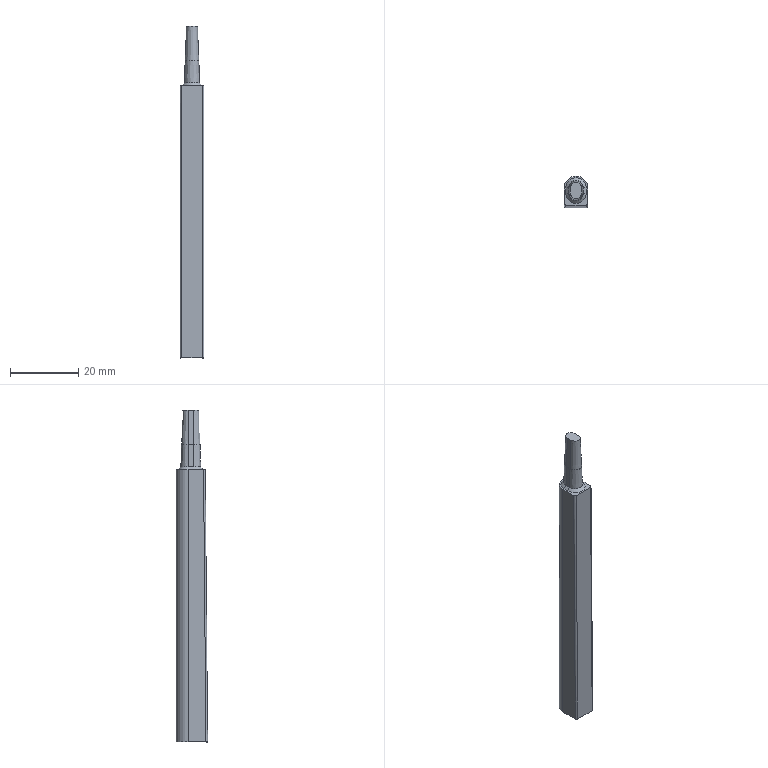Part | SolidWorks | features BaseBody 1 | 1 solid | 22 faces | box 7 x 9.198 x 97.496 mm | volume 4841 mm3 | plane 13 | cone 6 | cylinder 3 | commonest cylinder face diameters 1 x2 7 x1
STEP:
#1=CARTESIAN_POINT('',(-166.55,-32.434,17.496));
#2=VERTEX_POINT('',#1);
#3=CARTESIAN_POINT('',(-169.79,-32.434,17.496));
#4=VERTEX_POINT('',#3);
#5=CARTESIAN_POINT('',(-168.17,-32.434,17.496));
#6=DIRECTION('',(0.,0.,1.));
#7=DIRECTION('',(1.,0.,0.));
#8=AXIS2_PLACEMENT_3D('',#5,#6,#7);
#9=CIRCLE('',#8,1.62);
#10=EDGE_CURVE('',#2,#4,#9,.T.);
#11=ORIENTED_EDGE('',*,*,#10,.T.);
#12=CARTESIAN_POINT('',(-169.79,-33.942,17.496));
#13=VERTEX_POINT('',#12);
#14=CARTESIAN_POINT('',(-169.79,-33.188,17.496));
#15=DIRECTION('',(0.,-1.,0.));
#16=VECTOR('',#15,1000.);
#17=LINE('',#14,#16);
#18=EDGE_CURVE('',#4,#13,#17,.T.);
#19=ORIENTED_EDGE('',*,*,#18,.T.);
#20=CARTESIAN_POINT('',(-166.55,-33.942,17.496));
#21=VERTEX_POINT('',#20);
#22=CARTESIAN_POINT('',(-168.17,-33.942,17.496));
#23=DIRECTION('',(0.,0.,1.));
#24=DIRECTION('',(1.,0.,0.));
#25=AXIS2_PLACEMENT_3D('',#22,#23,#24);
#26=CIRCLE('',#25,1.62);
#27=EDGE_CURVE('',#13,#21,#26,.T.);
#28=ORIENTED_EDGE('',*,*,#27,.T.);
#29=CARTESIAN_POINT('',(-166.55,-33.188,17.496));
#30=DIRECTION('',(0.,1.,0.));
#31=VECTOR('',#30,1000.);
#32=LINE('',#29,#31);
#33=EDGE_CURVE('',#21,#2,#32,.T.);
#34=ORIENTED_EDGE('',*,*,#33,.T.);
#35=EDGE_LOOP('',(#11,#19,#28,#34));
#36=FACE_OUTER_BOUND('',#35,.T.);
#37=CARTESIAN_POINT('',(-178.728,104.314,17.496));
#38=DIRECTION('',(0.,0.,-1.));
#39=DIRECTION('',(1.,0.,0.));
#40=AXIS2_PLACEMENT_3D('',#37,#38,#39);
#41=PLANE('',#40);
#42=ADVANCED_FACE('',(#36),#41,.F.);
#43=CARTESIAN_POINT('',(-166.199,-33.942,7.441));
#44=VERTEX_POINT('',#43);
#45=CARTESIAN_POINT('',(-166.209,-33.942,7.732));
#46=DIRECTION('',(-0.0349,0.,0.9994));
#47=VECTOR('',#46,1000.);
#48=LINE('',#45,#47);
#49=EDGE_CURVE('',#44,#21,#48,.T.);
#50=ORIENTED_EDGE('',*,*,#49,.F.);
#51=CARTESIAN_POINT('',(-166.199,-32.434,7.441));
#52=VERTEX_POINT('',#51);
#53=CARTESIAN_POINT('',(-166.199,104.314,7.441));
#54=DIRECTION('',(0.,-1.,0.));
#55=VECTOR('',#54,1000.);
#56=LINE('',#53,#55);
#57=EDGE_CURVE('',#52,#44,#56,.T.);
#58=ORIENTED_EDGE('',*,*,#57,.F.);
#59=CARTESIAN_POINT('',(-166.209,-32.434,7.732));
#60=DIRECTION('',(-0.0349,0.,0.9994));
#61=VECTOR('',#60,1000.);
#62=LINE('',#59,#61);
#63=EDGE_CURVE('',#52,#2,#62,.T.);
#64=ORIENTED_EDGE('',*,*,#63,.T.);
#65=ORIENTED_EDGE('',*,*,#33,.F.);
#66=EDGE_LOOP('',(#50,#58,#64,#65));
#67=FACE_OUTER_BOUND('',#66,.T.);
#68=CARTESIAN_POINT('',(-166.209,-33.188,7.732));
#69=DIRECTION('',(-0.9994,0.,-0.0349));
#70=DIRECTION('',(0.0349,0.,-0.9994));
#71=AXIS2_PLACEMENT_3D('',#68,#69,#70);
#72=PLANE('',#71);
#73=ADVANCED_FACE('',(#67),#72,.F.);
#74=ORIENTED_EDGE('',*,*,#63,.F.);
#75=CARTESIAN_POINT('',(-170.141,-32.434,7.441));
#76=VERTEX_POINT('',#75);
#77=CARTESIAN_POINT('',(-168.17,-32.434,7.441));
#78=DIRECTION('',(0.,0.,-1.));
#79=DIRECTION('',(1.,0.,0.));
#80=AXIS2_PLACEMENT_3D('',#77,#78,#79);
#81=CIRCLE('',#80,1.971);
#82=EDGE_CURVE('',#76,#52,#81,.T.);
#83=ORIENTED_EDGE('',*,*,#82,.F.);
#84=CARTESIAN_POINT('',(-170.131,-32.434,7.732));
#85=DIRECTION('',(0.0349,0.,0.9994));
#86=VECTOR('',#85,1000.);
#87=LINE('',#84,#86);
#88=EDGE_CURVE('',#76,#4,#87,.T.);
#89=ORIENTED_EDGE('',*,*,#88,.T.);
#90=ORIENTED_EDGE('',*,*,#10,.F.);
#91=EDGE_LOOP('',(#74,#83,#89,#90));
#92=FACE_OUTER_BOUND('',#91,.T.);
#93=CARTESIAN_POINT('',(-168.17,-32.434,7.732));
#94=DIRECTION('',(0.,0.,-1.));
#95=DIRECTION('',(1.,0.,0.));
#96=AXIS2_PLACEMENT_3D('',#93,#94,#95);
#97=CONICAL_SURFACE('',#96,1.961,0.03491);
#98=ADVANCED_FACE('',(#92),#97,.T.);
#99=ORIENTED_EDGE('',*,*,#88,.F.);
#100=CARTESIAN_POINT('',(-170.141,-33.942,7.441));
#101=VERTEX_POINT('',#100);
#102=CARTESIAN_POINT('',(-170.141,104.314,7.441));
#103=DIRECTION('',(0.,1.,0.));
#104=VECTOR('',#103,1000.);
#105=LINE('',#102,#104);
#106=EDGE_CURVE('',#101,#76,#105,.T.);
#107=ORIENTED_EDGE('',*,*,#106,.F.);
#108=CARTESIAN_POINT('',(-170.131,-33.942,7.732));
#109=DIRECTION('',(0.0349,0.,0.9994));
#110=VECTOR('',#109,1000.);
#111=LINE('',#108,#110);
#112=EDGE_CURVE('',#101,#13,#111,.T.);
#113=ORIENTED_EDGE('',*,*,#112,.T.);
#114=ORIENTED_EDGE('',*,*,#18,.F.);
#115=EDGE_LOOP('',(#99,#107,#113,#114));
#116=FACE_OUTER_BOUND('',#115,.T.);
#117=CARTESIAN_POINT('',(-170.131,-33.188,7.732));
#118=DIRECTION('',(0.9994,0.,-0.0349));
#119=DIRECTION('',(0.0349,0.,0.9994));
#120=AXIS2_PLACEMENT_3D('',#117,#118,#119);
#121=PLANE('',#120);
#122=ADVANCED_FACE('',(#116),#121,.F.);
#123=ORIENTED_EDGE('',*,*,#112,.F.);
#124=CARTESIAN_POINT('',(-168.17,-33.942,7.441));
#125=DIRECTION('',(0.,0.,-1.));
#126=DIRECTION('',(1.,0.,0.));
#127=AXIS2_PLACEMENT_3D('',#124,#125,#126);
#128=CIRCLE('',#127,1.971);
#129=EDGE_CURVE('',#44,#101,#128,.T.);
#130=ORIENTED_EDGE('',*,*,#129,.F.);
#131=ORIENTED_EDGE('',*,*,#49,.T.);
#132=ORIENTED_EDGE('',*,*,#27,.F.);
#133=EDGE_LOOP('',(#123,#130,#131,#132));
#134=FACE_OUTER_BOUND('',#133,.T.);
#135=CARTESIAN_POINT('',(-168.17,-33.942,7.732));
#136=DIRECTION('',(0.,0.,-1.));
#137=DIRECTION('',(1.,0.,0.));
#138=AXIS2_PLACEMENT_3D('',#135,#136,#137);
#139=CONICAL_SURFACE('',#138,1.961,0.03491);
#140=ADVANCED_FACE('',(#134),#139,.T.);
#141=CARTESIAN_POINT('',(-170.187,-33.942,7.441));
#142=VERTEX_POINT('',#141);
#143=CARTESIAN_POINT('',(-170.187,-32.434,7.441));
#144=VERTEX_POINT('',#143);
#145=CARTESIAN_POINT('',(-170.187,104.314,7.441));
#146=DIRECTION('',(0.,1.,0.));
#147=VECTOR('',#146,1000.);
#148=LINE('',#145,#147);
#149=EDGE_CURVE('',#142,#144,#148,.T.);
#150=ORIENTED_EDGE('',*,*,#149,.F.);
#151=CARTESIAN_POINT('',(-166.153,-33.942,7.441));
#152=VERTEX_POINT('',#151);
#153=CARTESIAN_POINT('',(-168.17,-33.942,7.441));
#154=DIRECTION('',(0.,0.,-1.));
#155=DIRECTION('',(1.,0.,0.));
#156=AXIS2_PLACEMENT_3D('',#153,#154,#155);
#157=CIRCLE('',#156,2.017);
#158=EDGE_CURVE('',#152,#142,#157,.T.);
#159=ORIENTED_EDGE('',*,*,#158,.F.);
#160=CARTESIAN_POINT('',(-166.153,-32.434,7.441));
#161=VERTEX_POINT('',#160);
#162=CARTESIAN_POINT('',(-166.153,104.314,7.441));
#163=DIRECTION('',(0.,-1.,0.));
#164=VECTOR('',#163,1000.);
#165=LINE('',#162,#164);
#166=EDGE_CURVE('',#161,#152,#165,.T.);
#167=ORIENTED_EDGE('',*,*,#166,.F.);
#168=CARTESIAN_POINT('',(-168.17,-32.434,7.441));
#169=DIRECTION('',(0.,0.,-1.));
#170=DIRECTION('',(1.,0.,0.));
#171=AXIS2_PLACEMENT_3D('',#168,#169,#170);
#172=CIRCLE('',#171,2.017);
#173=EDGE_CURVE('',#144,#161,#172,.T.);
#174=ORIENTED_EDGE('',*,*,#173,.F.);
#175=EDGE_LOOP('',(#150,#159,#167,#174));
#176=FACE_OUTER_BOUND('',#175,.T.);
#177=ORIENTED_EDGE('',*,*,#129,.T.);
#178=ORIENTED_EDGE('',*,*,#106,.T.);
#179=ORIENTED_EDGE('',*,*,#82,.T.);
#180=ORIENTED_EDGE('',*,*,#57,.T.);
#181=EDGE_LOOP('',(#177,#178,#179,#180));
#182=FACE_BOUND('',#181,.T.);
#183=CARTESIAN_POINT('',(-178.728,104.314,7.441));
#184=DIRECTION('',(0.,0.,-1.));
#185=DIRECTION('',(1.,0.,0.));
#186=AXIS2_PLACEMENT_3D('',#183,#184,#185);
#187=PLANE('',#186);
#188=ADVANCED_FACE('',(#176,#182),#187,.F.);
#189=CARTESIAN_POINT('',(-170.361,-32.434,0.8042));
#190=VERTEX_POINT('',#189);
#191=CARTESIAN_POINT('',(-170.382,-32.434,-0.007896));
#192=DIRECTION('',(0.02618,0.,0.9997));
#193=VECTOR('',#192,1000.);
#194=LINE('',#191,#193);
#195=EDGE_CURVE('',#190,#144,#194,.T.);
#196=ORIENTED_EDGE('',*,*,#195,.T.);
#197=ORIENTED_EDGE('',*,*,#173,.T.);
#198=CARTESIAN_POINT('',(-165.979,-32.434,0.8042));
#199=VERTEX_POINT('',#198);
#200=CARTESIAN_POINT('',(-165.958,-32.434,-0.007896));
#201=DIRECTION('',(-0.02618,0.000000001,0.9997));
#202=VECTOR('',#201,1000.);
#203=LINE('',#200,#202);
#204=EDGE_CURVE('',#199,#161,#203,.T.);
#205=ORIENTED_EDGE('',*,*,#204,.F.);
#206=CARTESIAN_POINT('',(-168.17,-32.434,0.8042));
#207=DIRECTION('',(0.,0.,-1.));
#208=DIRECTION('',(-1.,0.,0.));
#209=AXIS2_PLACEMENT_3D('',#206,#207,#208);
#210=CIRCLE('',#209,2.191);
#211=EDGE_CURVE('',#190,#199,#210,.T.);
#212=ORIENTED_EDGE('',*,*,#211,.F.);
#213=EDGE_LOOP('',(#196,#197,#205,#212));
#214=FACE_OUTER_BOUND('',#213,.T.);
#215=CARTESIAN_POINT('',(-168.17,-32.434,-0.007896));
#216=DIRECTION('',(0.,0.,-1.));
#217=DIRECTION('',(1.,0.,0.));
#218=AXIS2_PLACEMENT_3D('',#215,#216,#217);
#219=CONICAL_SURFACE('',#218,2.212,0.02618);
#220=ADVANCED_FACE('',(#214),#219,.T.);
#221=CARTESIAN_POINT('',(-170.361,-33.942,0.8042));
#222=VERTEX_POINT('',#221);
#223=CARTESIAN_POINT('',(-170.382,-33.942,-0.007896));
#224=DIRECTION('',(0.02618,-0.000000001,0.9997));
#225=VECTOR('',#224,1000.);
#226=LINE('',#223,#225);
#227=EDGE_CURVE('',#222,#142,#226,.T.);
#228=ORIENTED_EDGE('',*,*,#227,.T.);
#229=ORIENTED_EDGE('',*,*,#149,.T.);
#230=ORIENTED_EDGE('',*,*,#195,.F.);
#231=CARTESIAN_POINT('',(-170.361,24.12,0.8042));
#232=DIRECTION('',(0.,1.,0.));
#233=VECTOR('',#232,1000.);
#234=LINE('',#231,#233);
#235=EDGE_CURVE('',#222,#190,#234,.T.);
#236=ORIENTED_EDGE('',*,*,#235,.F.);
#237=EDGE_LOOP('',(#228,#229,#230,#236));
#238=FACE_OUTER_BOUND('',#237,.T.);
#239=CARTESIAN_POINT('',(-170.382,24.12,-0.007896));
#240=DIRECTION('',(0.9997,0.,-0.02618));
#241=DIRECTION('',(0.02618,0.,0.9997));
#242=AXIS2_PLACEMENT_3D('',#239,#240,#241);
#243=PLANE('',#242);
#244=ADVANCED_FACE('',(#238),#243,.F.);
#245=CARTESIAN_POINT('',(-165.979,-33.942,0.8042));
#246=VERTEX_POINT('',#245);
#247=CARTESIAN_POINT('',(-165.958,-33.942,-0.007896));
#248=DIRECTION('',(-0.02618,0.,0.9997));
#249=VECTOR('',#248,1000.);
#250=LINE('',#247,#249);
#251=EDGE_CURVE('',#246,#152,#250,.T.);
#252=ORIENTED_EDGE('',*,*,#251,.T.);
#253=ORIENTED_EDGE('',*,*,#158,.T.);
#254=ORIENTED_EDGE('',*,*,#227,.F.);
#255=CARTESIAN_POINT('',(-168.17,-33.942,0.8042));
#256=DIRECTION('',(0.,0.,-1.));
#257=DIRECTION('',(-1.,0.,0.));
#258=AXIS2_PLACEMENT_3D('',#255,#256,#257);
#259=CIRCLE('',#258,2.191);
#260=EDGE_CURVE('',#246,#222,#259,.T.);
#261=ORIENTED_EDGE('',*,*,#260,.F.);
#262=EDGE_LOOP('',(#252,#253,#254,#261));
#263=FACE_OUTER_BOUND('',#262,.T.);
#264=CARTESIAN_POINT('',(-168.17,-33.942,-0.007896));
#265=DIRECTION('',(0.,0.,-1.));
#266=DIRECTION('',(1.,0.,0.));
#267=AXIS2_PLACEMENT_3D('',#264,#265,#266);
#268=CONICAL_SURFACE('',#267,2.212,0.02618);
#269=ADVANCED_FACE('',(#263),#268,.T.);
#270=ORIENTED_EDGE('',*,*,#204,.T.);
#271=ORIENTED_EDGE('',*,*,#166,.T.);
#272=ORIENTED_EDGE('',*,*,#251,.F.);
#273=CARTESIAN_POINT('',(-165.979,24.12,0.8042));
#274=DIRECTION('',(0.,-1.,0.));
#275=VECTOR('',#274,1000.);
#276=LINE('',#273,#275);
#277=EDGE_CURVE('',#199,#246,#276,.T.);
#278=ORIENTED_EDGE('',*,*,#277,.F.);
#279=EDGE_LOOP('',(#270,#271,#272,#278));
#280=FACE_OUTER_BOUND('',#279,.T.);
#281=CARTESIAN_POINT('',(-165.958,24.12,-0.007896));
#282=DIRECTION('',(-0.9997,0.,-0.02618));
#283=DIRECTION('',(0.02618,0.,-0.9997));
#284=AXIS2_PLACEMENT_3D('',#281,#282,#283);
#285=PLANE('',#284);
#286=ADVANCED_FACE('',(#280),#285,.F.);
#287=CARTESIAN_POINT('',(-165.153,-32.434,0.));
#288=VERTEX_POINT('',#287);
#289=CARTESIAN_POINT('',(-165.153,-32.434,0.));
#290=DIRECTION('',(-0.7163,0.,0.6978));
#291=VECTOR('',#290,1000.);
#292=LINE('',#289,#291);
#293=EDGE_CURVE('',#288,#199,#292,.T.);
#294=ORIENTED_EDGE('',*,*,#293,.F.);
#295=CARTESIAN_POINT('',(-171.186,-32.434,0.));
#296=VERTEX_POINT('',#295);
#297=CARTESIAN_POINT('',(-168.17,-32.434,0.));
#298=DIRECTION('',(0.,0.,1.));
#299=DIRECTION('',(1.,0.,0.));
#300=AXIS2_PLACEMENT_3D('',#297,#298,#299);
#301=CIRCLE('',#300,3.017);
#302=EDGE_CURVE('',#288,#296,#301,.T.);
#303=ORIENTED_EDGE('',*,*,#302,.T.);
#304=CARTESIAN_POINT('',(-171.186,-32.434,0.));
#305=DIRECTION('',(0.7163,0.,0.6978));
#306=VECTOR('',#305,1000.);
#307=LINE('',#304,#306);
#308=EDGE_CURVE('',#296,#190,#307,.T.);
#309=ORIENTED_EDGE('',*,*,#308,.T.);
#310=ORIENTED_EDGE('',*,*,#211,.T.);
#311=EDGE_LOOP('',(#294,#303,#309,#310));
#312=FACE_OUTER_BOUND('',#311,.T.);
#313=CARTESIAN_POINT('',(-168.17,-32.434,0.5026));
#314=DIRECTION('',(0.,0.,-1.));
#315=DIRECTION('',(1.,0.,0.));
#316=AXIS2_PLACEMENT_3D('',#313,#314,#315);
#317=CONICAL_SURFACE('',#316,2.501,0.7985);
#318=ADVANCED_FACE('',(#312),#317,.T.);
#319=CARTESIAN_POINT('',(-171.186,-33.942,0.));
#320=VERTEX_POINT('',#319);
#321=CARTESIAN_POINT('',(-170.67,-33.942,0.5026));
#322=DIRECTION('',(-0.7163,0.,-0.6978));
#323=VECTOR('',#322,1000.);
#324=LINE('',#321,#323);
#325=EDGE_CURVE('',#222,#320,#324,.T.);
#326=ORIENTED_EDGE('',*,*,#325,.F.);
#327=ORIENTED_EDGE('',*,*,#235,.T.);
#328=ORIENTED_EDGE('',*,*,#308,.F.);
#329=CARTESIAN_POINT('',(-171.186,-33.942,0.));
#330=DIRECTION('',(0.,-1.,0.));
#331=VECTOR('',#330,1000.);
#332=LINE('',#329,#331);
#333=EDGE_CURVE('',#296,#320,#332,.T.);
#334=ORIENTED_EDGE('',*,*,#333,.T.);
#335=EDGE_LOOP('',(#326,#327,#328,#334));
#336=FACE_OUTER_BOUND('',#335,.T.);
#337=CARTESIAN_POINT('',(-170.67,24.12,0.5026));
#338=DIRECTION('',(-0.6978,0.,0.7163));
#339=DIRECTION('',(-0.7163,0.,-0.6978));
#340=AXIS2_PLACEMENT_3D('',#337,#338,#339);
#341=PLANE('',#340);
#342=ADVANCED_FACE('',(#336),#341,.T.);
#343=CARTESIAN_POINT('',(-165.153,-33.942,0.));
#344=VERTEX_POINT('',#343);
#345=CARTESIAN_POINT('',(-165.669,-33.942,0.5026));
#346=DIRECTION('',(0.7163,-0.000000006,-0.6978));
#347=VECTOR('',#346,1000.);
#348=LINE('',#345,#347);
#349=EDGE_CURVE('',#246,#344,#348,.T.);
#350=ORIENTED_EDGE('',*,*,#349,.F.);
#351=ORIENTED_EDGE('',*,*,#260,.T.);
#352=ORIENTED_EDGE('',*,*,#325,.T.);
#353=CARTESIAN_POINT('',(-168.17,-33.942,0.));
#354=DIRECTION('',(0.,0.,1.));
#355=DIRECTION('',(1.,0.,0.));
#356=AXIS2_PLACEMENT_3D('',#353,#354,#355);
#357=CIRCLE('',#356,3.017);
#358=EDGE_CURVE('',#320,#344,#357,.T.);
#359=ORIENTED_EDGE('',*,*,#358,.T.);
#360=EDGE_LOOP('',(#350,#351,#352,#359));
#361=FACE_OUTER_BOUND('',#360,.T.);
#362=CARTESIAN_POINT('',(-168.17,-33.942,0.5026));
#363=DIRECTION('',(0.,0.,-1.));
#364=DIRECTION('',(1.,0.,0.));
#365=AXIS2_PLACEMENT_3D('',#362,#363,#364);
#366=CONICAL_SURFACE('',#365,2.501,0.7985);
#367=ADVANCED_FACE('',(#361),#366,.T.);
#368=ORIENTED_EDGE('',*,*,#293,.T.);
#369=ORIENTED_EDGE('',*,*,#277,.T.);
#370=ORIENTED_EDGE('',*,*,#349,.T.);
#371=CARTESIAN_POINT('',(-165.153,-32.434,0.));
#372=DIRECTION('',(0.,1.,0.));
#373=VECTOR('',#372,1000.);
#374=LINE('',#371,#373);
#375=EDGE_CURVE('',#344,#288,#374,.T.);
#376=ORIENTED_EDGE('',*,*,#375,.T.);
#377=EDGE_LOOP('',(#368,#369,#370,#376));
#378=FACE_OUTER_BOUND('',#377,.T.);
#379=CARTESIAN_POINT('',(-165.669,24.12,0.5026));
#380=DIRECTION('',(0.6978,0.,0.7163));
#381=DIRECTION('',(-0.7163,0.,0.6978));
#382=AXIS2_PLACEMENT_3D('',#379,#380,#381);
#383=PLANE('',#382);
#384=ADVANCED_FACE('',(#378),#383,.T.);
#385=ORIENTED_EDGE('',*,*,#375,.F.);
#386=ORIENTED_EDGE('',*,*,#358,.F.);
#387=ORIENTED_EDGE('',*,*,#333,.F.);
#388=ORIENTED_EDGE('',*,*,#302,.F.);
#389=EDGE_LOOP('',(#385,#386,#387,#388));
#390=FACE_BOUND('',#389,.T.);
#391=CARTESIAN_POINT('',(-164.67,-32.434,0.));
#392=VERTEX_POINT('',#391);
#393=CARTESIAN_POINT('',(-164.67,-36.934,0.));
#394=VERTEX_POINT('',#393);
#395=CARTESIAN_POINT('',(-164.67,5.,0.));
#396=DIRECTION('',(0.,-1.,0.));
#397=VECTOR('',#396,1000.);
#398=LINE('',#395,#397);
#399=EDGE_CURVE('',#392,#394,#398,.T.);
#400=ORIENTED_EDGE('',*,*,#399,.F.);
#401=CARTESIAN_POINT('',(-171.67,-32.434,0.));
#402=VERTEX_POINT('',#401);
#403=CARTESIAN_POINT('',(-168.17,-32.434,0.));
#404=DIRECTION('',(0.,0.,-1.));
#405=DIRECTION('',(1.,0.,0.));
#406=AXIS2_PLACEMENT_3D('',#403,#404,#405);
#407=CIRCLE('',#406,3.5);
#408=EDGE_CURVE('',#402,#392,#407,.T.);
#409=ORIENTED_EDGE('',*,*,#408,.F.);
#410=CARTESIAN_POINT('',(-171.67,-36.934,0.));
#411=VERTEX_POINT('',#410);
#412=CARTESIAN_POINT('',(-171.67,5.,0.));
#413=DIRECTION('',(0.,1.,0.));
#414=VECTOR('',#413,1000.);
#415=LINE('',#412,#414);
#416=EDGE_CURVE('',#411,#402,#415,.T.);
#417=ORIENTED_EDGE('',*,*,#416,.F.);
#418=CARTESIAN_POINT('',(-171.17,-37.434,0.));
#419=VERTEX_POINT('',#418);
#420=CARTESIAN_POINT('',(-171.67,-36.934,0.));
#421=CARTESIAN_POINT('',(-171.67,-37.226,0.));
#422=CARTESIAN_POINT('',(-171.463,-37.434,0.));
#423=CARTESIAN_POINT('',(-171.17,-37.434,0.));
#424=(BOUNDED_CURVE()B_SPLINE_CURVE(3,(#420,#421,#422,#423),.UNSPECIFIED.,.F.,.F.)B_SPLINE_CURVE_WITH_KNOTS((4,4),(1.571,3.142),.UNSPECIFIED.)CURVE()GEOMETRIC_REPRESENTATION_ITEM()RATIONAL_B_SPLINE_CURVE((1.,0.8047,0.8047,1.))REPRESENTATION_ITEM(''));
#425=EDGE_CURVE('',#411,#419,#424,.T.);
#426=ORIENTED_EDGE('',*,*,#425,.T.);
#427=CARTESIAN_POINT('',(-165.17,-37.434,0.));
#428=VERTEX_POINT('',#427);
#429=CARTESIAN_POINT('',(0.,-37.434,0.));
#430=DIRECTION('',(-1.,0.,0.));
#431=VECTOR('',#430,1000.);
#432=LINE('',#429,#431);
#433=EDGE_CURVE('',#428,#419,#432,.T.);
#434=ORIENTED_EDGE('',*,*,#433,.F.);
#435=CARTESIAN_POINT('',(-165.17,-37.434,0.));
#436=CARTESIAN_POINT('',(-164.877,-37.434,0.));
#437=CARTESIAN_POINT('',(-164.67,-37.226,0.));
#438=CARTESIAN_POINT('',(-164.67,-36.934,0.));
#439=(BOUNDED_CURVE()B_SPLINE_CURVE(3,(#435,#436,#437,#438),.UNSPECIFIED.,.F.,.F.)B_SPLINE_CURVE_WITH_KNOTS((4,4),(3.142,4.712),.UNSPECIFIED.)CURVE()GEOMETRIC_REPRESENTATION_ITEM()RATIONAL_B_SPLINE_CURVE((1.,0.8047,0.8047,1.))REPRESENTATION_ITEM(''));
#440=EDGE_CURVE('',#428,#394,#439,.T.);
#441=ORIENTED_EDGE('',*,*,#440,.T.);
#442=EDGE_LOOP('',(#400,#409,#417,#426,#434,#441));
#443=FACE_OUTER_BOUND('',#442,.T.);
#444=CARTESIAN_POINT('',(0.,5.,0.));
#445=DIRECTION('',(0.,0.,1.));
#446=DIRECTION('',(1.,0.,0.));
#447=AXIS2_PLACEMENT_3D('',#444,#445,#446);
#448=PLANE('',#447);
#449=ADVANCED_FACE('',(#390,#443),#448,.T.);
#450=CARTESIAN_POINT('',(-171.67,-37.632,-80.));
#451=VERTEX_POINT('',#450);
#452=CARTESIAN_POINT('',(-171.67,-36.671,30.037));
#453=DIRECTION('',(0.,0.008727,1.));
#454=VECTOR('',#453,1000.);
#455=LINE('',#452,#454);
#456=EDGE_CURVE('',#451,#411,#455,.T.);
#457=ORIENTED_EDGE('',*,*,#456,.T.);
#458=ORIENTED_EDGE('',*,*,#416,.T.);
#459=CARTESIAN_POINT('',(-171.67,-32.434,-80.));
#460=VERTEX_POINT('',#459);
#461=CARTESIAN_POINT('',(-171.67,-32.434,30.));
#462=DIRECTION('',(0.,0.,-1.));
#463=VECTOR('',#462,1000.);
#464=LINE('',#461,#463);
#465=EDGE_CURVE('',#402,#460,#464,.T.);
#466=ORIENTED_EDGE('',*,*,#465,.T.);
#467=CARTESIAN_POINT('',(-171.67,-32.434,-80.));
#468=DIRECTION('',(0.,-1.,0.));
#469=VECTOR('',#468,1000.);
#470=LINE('',#467,#469);
#471=EDGE_CURVE('',#460,#451,#470,.T.);
#472=ORIENTED_EDGE('',*,*,#471,.T.);
#473=EDGE_LOOP('',(#457,#458,#466,#472));
#474=FACE_OUTER_BOUND('',#473,.T.);
#475=CARTESIAN_POINT('',(-171.67,-32.434,30.));
#476=DIRECTION('',(1.,0.,0.));
#477=DIRECTION('',(0.,0.,-1.));
#478=AXIS2_PLACEMENT_3D('',#475,#476,#477);
#479=PLANE('',#478);
#480=ADVANCED_FACE('',(#474),#479,.F.);
#481=CARTESIAN_POINT('',(-165.17,-38.132,-80.));
#482=VERTEX_POINT('',#481);
#483=CARTESIAN_POINT('',(-165.17,-37.434,0.));
#484=DIRECTION('',(0.,0.008727,1.));
#485=VECTOR('',#484,1000.);
#486=LINE('',#483,#485);
#487=EDGE_CURVE('',#482,#428,#486,.T.);
#488=ORIENTED_EDGE('',*,*,#487,.T.);
#489=ORIENTED_EDGE('',*,*,#433,.T.);
#490=CARTESIAN_POINT('',(-171.17,-38.132,-80.));
#491=VERTEX_POINT('',#490);
#492=CARTESIAN_POINT('',(-171.17,-37.434,0.));
#493=DIRECTION('',(0.,-0.008727,-1.));
#494=VECTOR('',#493,1000.);
#495=LINE('',#492,#494);
#496=EDGE_CURVE('',#419,#491,#495,.T.);
#497=ORIENTED_EDGE('',*,*,#496,.T.);
#498=CARTESIAN_POINT('',(-168.17,-38.132,-80.));
#499=DIRECTION('',(1.,0.,0.));
#500=VECTOR('',#499,1000.);
#501=LINE('',#498,#500);
#502=EDGE_CURVE('',#491,#482,#501,.T.);
#503=ORIENTED_EDGE('',*,*,#502,.T.);
#504=EDGE_LOOP('',(#488,#489,#497,#503));
#505=FACE_OUTER_BOUND('',#504,.T.);
#506=CARTESIAN_POINT('',(-168.17,-37.434,0.));
#507=DIRECTION('',(0.,-1.,0.008727));
#508=DIRECTION('',(0.,-0.008727,-1.));
#509=AXIS2_PLACEMENT_3D('',#506,#507,#508);
#510=PLANE('',#509);
#511=ADVANCED_FACE('',(#505),#510,.T.);
#512=CARTESIAN_POINT('',(-164.67,-32.434,-80.));
#513=VERTEX_POINT('',#512);
#514=CARTESIAN_POINT('',(-164.67,-32.434,30.));
#515=DIRECTION('',(0.,0.,-1.));
#516=VECTOR('',#515,1000.);
#517=LINE('',#514,#516);
#518=EDGE_CURVE('',#392,#513,#517,.T.);
#519=ORIENTED_EDGE('',*,*,#518,.F.);
#520=ORIENTED_EDGE('',*,*,#399,.T.);
#521=CARTESIAN_POINT('',(-164.67,-37.632,-80.));
#522=VERTEX_POINT('',#521);
#523=CARTESIAN_POINT('',(-164.67,-36.672,29.993));
#524=DIRECTION('',(0.,-0.008727,-1.));
#525=VECTOR('',#524,1000.);
#526=LINE('',#523,#525);
#527=EDGE_CURVE('',#394,#522,#526,.T.);
#528=ORIENTED_EDGE('',*,*,#527,.T.);
#529=CARTESIAN_POINT('',(-164.67,-37.434,-80.));
#530=DIRECTION('',(0.,1.,0.));
#531=VECTOR('',#530,1000.);
#532=LINE('',#529,#531);
#533=EDGE_CURVE('',#522,#513,#532,.T.);
#534=ORIENTED_EDGE('',*,*,#533,.T.);
#535=EDGE_LOOP('',(#519,#520,#528,#534));
#536=FACE_OUTER_BOUND('',#535,.T.);
#537=CARTESIAN_POINT('',(-164.67,-37.434,30.));
#538=DIRECTION('',(-1.,0.,0.));
#539=DIRECTION('',(0.,0.,1.));
#540=AXIS2_PLACEMENT_3D('',#537,#538,#539);
#541=PLANE('',#540);
#542=ADVANCED_FACE('',(#536),#541,.F.);
#543=ORIENTED_EDGE('',*,*,#465,.F.);
#544=ORIENTED_EDGE('',*,*,#408,.T.);
#545=ORIENTED_EDGE('',*,*,#518,.T.);
#546=CARTESIAN_POINT('',(-168.17,-32.434,-80.));
#547=DIRECTION('',(0.,0.,1.));
#548=DIRECTION('',(1.,0.,0.));
#549=AXIS2_PLACEMENT_3D('',#546,#547,#548);
#550=CIRCLE('',#549,3.5);
#551=EDGE_CURVE('',#513,#460,#550,.T.);
#552=ORIENTED_EDGE('',*,*,#551,.T.);
#553=EDGE_LOOP('',(#543,#544,#545,#552));
#554=FACE_OUTER_BOUND('',#553,.T.);
#555=CARTESIAN_POINT('',(-168.17,-32.434,30.));
#556=DIRECTION('',(0.,0.,-1.));
#557=DIRECTION('',(-1.,0.,0.));
#558=AXIS2_PLACEMENT_3D('',#555,#556,#557);
#559=CYLINDRICAL_SURFACE('',#558,3.5);
#560=ADVANCED_FACE('',(#554),#559,.T.);
#561=ORIENTED_EDGE('',*,*,#440,.F.);
#562=ORIENTED_EDGE('',*,*,#487,.F.);
#563=CARTESIAN_POINT('',(-164.67,-37.632,-80.));
#564=CARTESIAN_POINT('',(-164.67,-37.925,-80.));
#565=CARTESIAN_POINT('',(-164.877,-38.132,-80.));
#566=CARTESIAN_POINT('',(-165.17,-38.132,-80.));
#567=(BOUNDED_CURVE()B_SPLINE_CURVE(3,(#563,#564,#565,#566),.UNSPECIFIED.,.F.,.F.)B_SPLINE_CURVE_WITH_KNOTS((4,4),(1.571,3.142),.UNSPECIFIED.)CURVE()GEOMETRIC_REPRESENTATION_ITEM()RATIONAL_B_SPLINE_CURVE((1.,0.8047,0.8047,1.))REPRESENTATION_ITEM(''));
#568=EDGE_CURVE('',#522,#482,#567,.T.);
#569=ORIENTED_EDGE('',*,*,#568,.F.);
#570=ORIENTED_EDGE('',*,*,#527,.F.);
#571=EDGE_LOOP('',(#561,#562,#569,#570));
#572=FACE_OUTER_BOUND('',#571,.T.);
#573=CARTESIAN_POINT('',(-165.17,-36.672,29.993));
#574=DIRECTION('',(0.,0.008727,1.));
#575=DIRECTION('',(0.,-1.,0.008727));
#576=AXIS2_PLACEMENT_3D('',#573,#574,#575);
#577=CYLINDRICAL_SURFACE('',#576,0.5);
#578=ADVANCED_FACE('',(#572),#577,.T.);
#579=ORIENTED_EDGE('',*,*,#425,.F.);
#580=ORIENTED_EDGE('',*,*,#456,.F.);
#581=CARTESIAN_POINT('',(-171.17,-38.132,-80.));
#582=CARTESIAN_POINT('',(-171.463,-38.132,-80.));
#583=CARTESIAN_POINT('',(-171.67,-37.925,-80.));
#584=CARTESIAN_POINT('',(-171.67,-37.632,-80.));
#585=(BOUNDED_CURVE()B_SPLINE_CURVE(3,(#581,#582,#583,#584),.UNSPECIFIED.,.F.,.T.)B_SPLINE_CURVE_WITH_KNOTS((4,4),(3.142,4.712),.UNSPECIFIED.)CURVE()GEOMETRIC_REPRESENTATION_ITEM()RATIONAL_B_SPLINE_CURVE((1.,0.8047,0.8047,1.))REPRESENTATION_ITEM(''));
#586=EDGE_CURVE('',#491,#451,#585,.T.);
#587=ORIENTED_EDGE('',*,*,#586,.F.);
#588=ORIENTED_EDGE('',*,*,#496,.F.);
#589=EDGE_LOOP('',(#579,#580,#587,#588));
#590=FACE_OUTER_BOUND('',#589,.T.);
#591=CARTESIAN_POINT('',(-171.17,-36.934,-0.004363));
#592=DIRECTION('',(0.,0.008727,1.));
#593=DIRECTION('',(0.,-1.,0.008727));
#594=AXIS2_PLACEMENT_3D('',#591,#592,#593);
#595=CYLINDRICAL_SURFACE('',#594,0.5);
#596=ADVANCED_FACE('',(#590),#595,.T.);
#597=ORIENTED_EDGE('',*,*,#533,.F.);
#598=ORIENTED_EDGE('',*,*,#568,.T.);
#599=ORIENTED_EDGE('',*,*,#502,.F.);
#600=ORIENTED_EDGE('',*,*,#586,.T.);
#601=ORIENTED_EDGE('',*,*,#471,.F.);
#602=ORIENTED_EDGE('',*,*,#551,.F.);
#603=EDGE_LOOP('',(#597,#598,#599,#600,#601,#602));
#604=FACE_OUTER_BOUND('',#603,.T.);
#605=CARTESIAN_POINT('',(-265.,-165.,-80.));
#606=DIRECTION('',(0.,0.,1.));
#607=DIRECTION('',(1.,0.,0.));
#608=AXIS2_PLACEMENT_3D('',#605,#606,#607);
#609=PLANE('',#608);
#610=ADVANCED_FACE('',(#604),#609,.F.);
#611=CLOSED_SHELL('',(#42,#73,#98,#122,#140,#188,#220,#244,#269,#286,#318,#342,#367,#384,#449,#480,#511,#542,#560,#578,#596,#610));
#612=MANIFOLD_SOLID_BREP('',#611);
#613=CARTESIAN_POINT('',(0.,0.,0.));
#614=DIRECTION('',(0.,0.,1.));
#615=DIRECTION('',(1.,0.,0.));
#616=AXIS2_PLACEMENT_3D('',#613,#614,#615);
#617=(LENGTH_UNIT()NAMED_UNIT(*)SI_UNIT(.MILLI.,.METRE.));
#618=UNCERTAINTY_MEASURE_WITH_UNIT(LENGTH_MEASURE(0.00001),#617,'','');
#619=(NAMED_UNIT(*)PLANE_ANGLE_UNIT()SI_UNIT($,.RADIAN.));
#620=(NAMED_UNIT(*)SI_UNIT($,.STERADIAN.)SOLID_ANGLE_UNIT());
#621=(GEOMETRIC_REPRESENTATION_CONTEXT(3)GLOBAL_UNCERTAINTY_ASSIGNED_CONTEXT((#618))GLOBAL_UNIT_ASSIGNED_CONTEXT((#617,#619,#620))REPRESENTATION_CONTEXT('',''));
#622=ADVANCED_BREP_SHAPE_REPRESENTATION('',(#612,#616),#621);